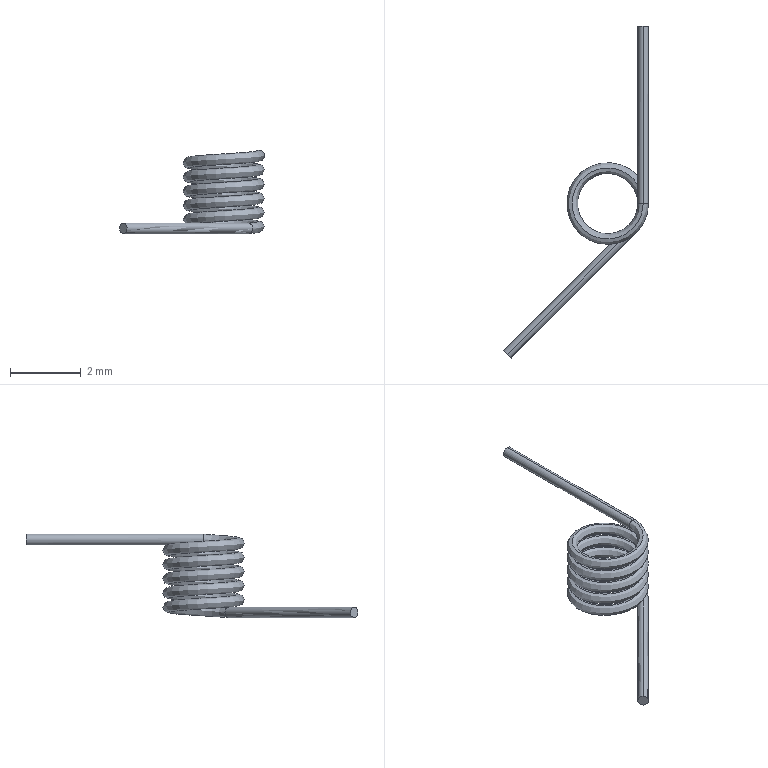Part | SolidWorks | features BaseBody 1, ICE 1 | 1 solid | 8 faces | box 4.085 x 9.349 x 2.35 mm | volume 2.987 mm3 | spline 4 | cylinder 2 | plane 2 | commonest cylinder face diameters 0.3 x2